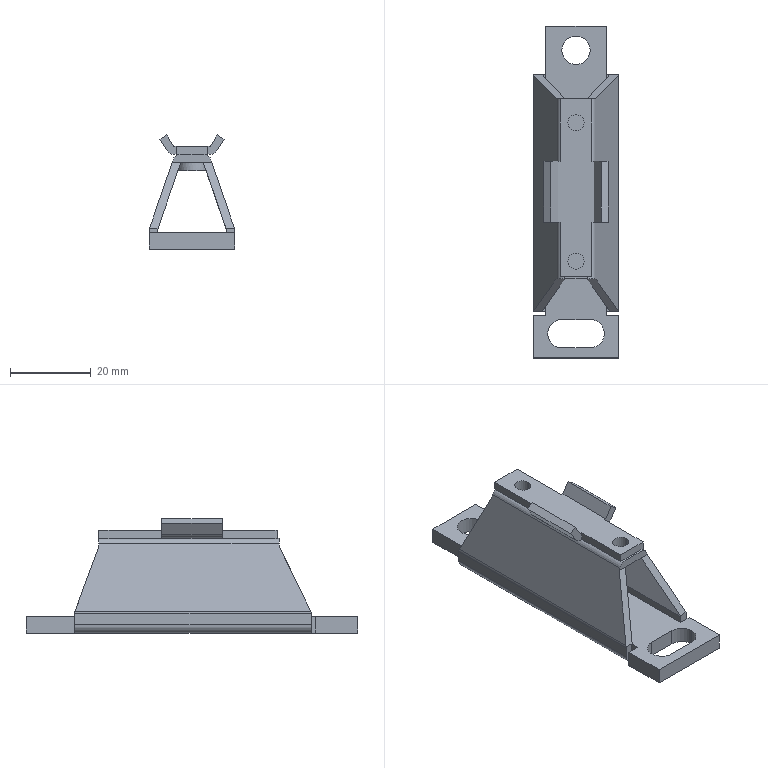Part | STEP file | Y300T_Y3035DB Rear Plate_3T | 1 solid | 76 faces | box 21 x 82 x 28.179 mm | volume 11258 mm3 | plane 54 | cylinder 22 | commonest cylinder face diameters 4 x12 7 x5 7.2 x5